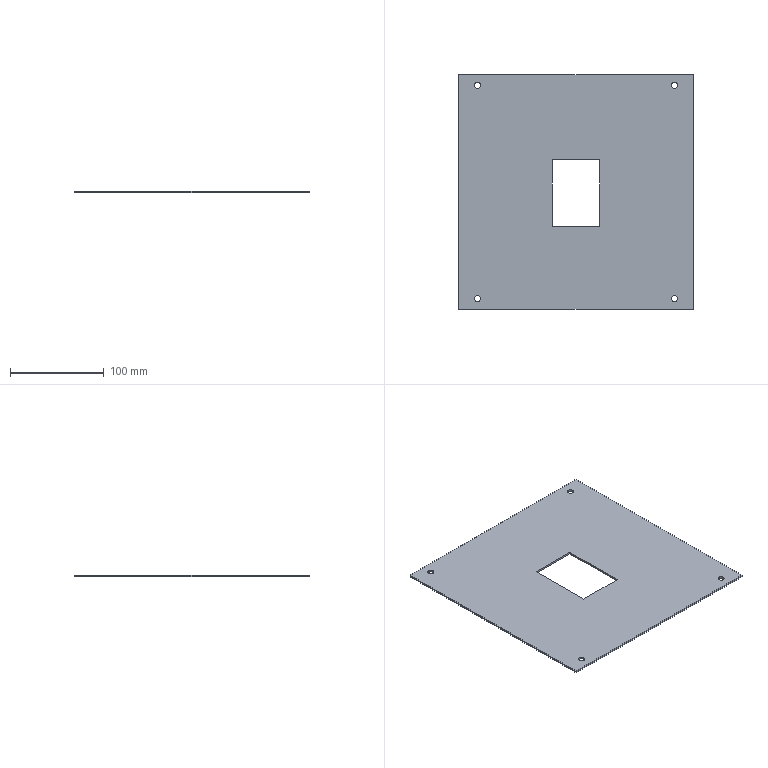Part | SolidWorks | features BaseBody 1 | 1 solid | 18 faces | box 250 x 250 x 2 mm | volume 117542 mm3 | plane 10 | cylinder 8 | commonest cylinder face diameters 6.5 x8
STEP:
#1=CARTESIAN_POINT('',(-108.25,113.5,-2.));
#2=VERTEX_POINT('',#1);
#3=CARTESIAN_POINT('',(-101.75,113.5,-2.));
#4=VERTEX_POINT('',#3);
#5=CARTESIAN_POINT('',(-105.,113.5,-2.));
#6=DIRECTION('',(0.,0.,1.));
#7=DIRECTION('',(1.,0.,0.));
#8=AXIS2_PLACEMENT_3D('',#5,#6,#7);
#9=CIRCLE('',#8,3.25);
#10=EDGE_CURVE('',#2,#4,#9,.T.);
#11=ORIENTED_EDGE('',*,*,#10,.F.);
#12=CARTESIAN_POINT('',(-108.25,113.5,0.));
#13=VERTEX_POINT('',#12);
#14=CARTESIAN_POINT('',(-108.25,113.5,-10.));
#15=DIRECTION('',(0.,0.,1.));
#16=VECTOR('',#15,1000.);
#17=LINE('',#14,#16);
#18=EDGE_CURVE('',#2,#13,#17,.T.);
#19=ORIENTED_EDGE('',*,*,#18,.T.);
#20=CARTESIAN_POINT('',(-101.75,113.5,0.));
#21=VERTEX_POINT('',#20);
#22=CARTESIAN_POINT('',(-105.,113.5,0.));
#23=DIRECTION('',(0.,0.,1.));
#24=DIRECTION('',(1.,0.,0.));
#25=AXIS2_PLACEMENT_3D('',#22,#23,#24);
#26=CIRCLE('',#25,3.25);
#27=EDGE_CURVE('',#13,#21,#26,.T.);
#28=ORIENTED_EDGE('',*,*,#27,.T.);
#29=CARTESIAN_POINT('',(-101.75,113.5,-10.));
#30=DIRECTION('',(0.,0.,1.));
#31=VECTOR('',#30,1000.);
#32=LINE('',#29,#31);
#33=EDGE_CURVE('',#4,#21,#32,.T.);
#34=ORIENTED_EDGE('',*,*,#33,.F.);
#35=EDGE_LOOP('',(#11,#19,#28,#34));
#36=FACE_OUTER_BOUND('',#35,.T.);
#37=CARTESIAN_POINT('',(-105.,113.5,-10.));
#38=DIRECTION('',(0.,0.,1.));
#39=DIRECTION('',(1.,0.,0.));
#40=AXIS2_PLACEMENT_3D('',#37,#38,#39);
#41=CYLINDRICAL_SURFACE('',#40,3.25);
#42=ADVANCED_FACE('',(#36),#41,.F.);
#43=CARTESIAN_POINT('',(101.75,113.5,-2.));
#44=VERTEX_POINT('',#43);
#45=CARTESIAN_POINT('',(108.25,113.5,-2.));
#46=VERTEX_POINT('',#45);
#47=CARTESIAN_POINT('',(105.,113.5,-2.));
#48=DIRECTION('',(0.,0.,1.));
#49=DIRECTION('',(1.,0.,0.));
#50=AXIS2_PLACEMENT_3D('',#47,#48,#49);
#51=CIRCLE('',#50,3.25);
#52=EDGE_CURVE('',#44,#46,#51,.T.);
#53=ORIENTED_EDGE('',*,*,#52,.F.);
#54=CARTESIAN_POINT('',(101.75,113.5,0.));
#55=VERTEX_POINT('',#54);
#56=CARTESIAN_POINT('',(101.75,113.5,-10.));
#57=DIRECTION('',(0.,0.,1.));
#58=VECTOR('',#57,1000.);
#59=LINE('',#56,#58);
#60=EDGE_CURVE('',#44,#55,#59,.T.);
#61=ORIENTED_EDGE('',*,*,#60,.T.);
#62=CARTESIAN_POINT('',(108.25,113.5,0.));
#63=VERTEX_POINT('',#62);
#64=CARTESIAN_POINT('',(105.,113.5,0.));
#65=DIRECTION('',(0.,0.,1.));
#66=DIRECTION('',(1.,0.,0.));
#67=AXIS2_PLACEMENT_3D('',#64,#65,#66);
#68=CIRCLE('',#67,3.25);
#69=EDGE_CURVE('',#55,#63,#68,.T.);
#70=ORIENTED_EDGE('',*,*,#69,.T.);
#71=CARTESIAN_POINT('',(108.25,113.5,-10.));
#72=DIRECTION('',(0.,0.,1.));
#73=VECTOR('',#72,1000.);
#74=LINE('',#71,#73);
#75=EDGE_CURVE('',#46,#63,#74,.T.);
#76=ORIENTED_EDGE('',*,*,#75,.F.);
#77=EDGE_LOOP('',(#53,#61,#70,#76));
#78=FACE_OUTER_BOUND('',#77,.T.);
#79=CARTESIAN_POINT('',(105.,113.5,-10.));
#80=DIRECTION('',(0.,0.,1.));
#81=DIRECTION('',(1.,0.,0.));
#82=AXIS2_PLACEMENT_3D('',#79,#80,#81);
#83=CYLINDRICAL_SURFACE('',#82,3.25);
#84=ADVANCED_FACE('',(#78),#83,.F.);
#85=CARTESIAN_POINT('',(101.75,-113.5,-2.));
#86=VERTEX_POINT('',#85);
#87=CARTESIAN_POINT('',(108.25,-113.5,-2.));
#88=VERTEX_POINT('',#87);
#89=CARTESIAN_POINT('',(105.,-113.5,-2.));
#90=DIRECTION('',(0.,0.,1.));
#91=DIRECTION('',(1.,0.,0.));
#92=AXIS2_PLACEMENT_3D('',#89,#90,#91);
#93=CIRCLE('',#92,3.25);
#94=EDGE_CURVE('',#86,#88,#93,.T.);
#95=ORIENTED_EDGE('',*,*,#94,.F.);
#96=CARTESIAN_POINT('',(101.75,-113.5,0.));
#97=VERTEX_POINT('',#96);
#98=CARTESIAN_POINT('',(101.75,-113.5,-10.));
#99=DIRECTION('',(0.,0.,1.));
#100=VECTOR('',#99,1000.);
#101=LINE('',#98,#100);
#102=EDGE_CURVE('',#86,#97,#101,.T.);
#103=ORIENTED_EDGE('',*,*,#102,.T.);
#104=CARTESIAN_POINT('',(108.25,-113.5,0.));
#105=VERTEX_POINT('',#104);
#106=CARTESIAN_POINT('',(105.,-113.5,0.));
#107=DIRECTION('',(0.,0.,1.));
#108=DIRECTION('',(1.,0.,0.));
#109=AXIS2_PLACEMENT_3D('',#106,#107,#108);
#110=CIRCLE('',#109,3.25);
#111=EDGE_CURVE('',#97,#105,#110,.T.);
#112=ORIENTED_EDGE('',*,*,#111,.T.);
#113=CARTESIAN_POINT('',(108.25,-113.5,-10.));
#114=DIRECTION('',(0.,0.,1.));
#115=VECTOR('',#114,1000.);
#116=LINE('',#113,#115);
#117=EDGE_CURVE('',#88,#105,#116,.T.);
#118=ORIENTED_EDGE('',*,*,#117,.F.);
#119=EDGE_LOOP('',(#95,#103,#112,#118));
#120=FACE_OUTER_BOUND('',#119,.T.);
#121=CARTESIAN_POINT('',(105.,-113.5,-10.));
#122=DIRECTION('',(0.,0.,1.));
#123=DIRECTION('',(1.,0.,0.));
#124=AXIS2_PLACEMENT_3D('',#121,#122,#123);
#125=CYLINDRICAL_SURFACE('',#124,3.25);
#126=ADVANCED_FACE('',(#120),#125,.F.);
#127=CARTESIAN_POINT('',(-108.25,-113.5,-2.));
#128=VERTEX_POINT('',#127);
#129=CARTESIAN_POINT('',(-101.75,-113.5,-2.));
#130=VERTEX_POINT('',#129);
#131=CARTESIAN_POINT('',(-105.,-113.5,-2.));
#132=DIRECTION('',(0.,0.,1.));
#133=DIRECTION('',(1.,0.,0.));
#134=AXIS2_PLACEMENT_3D('',#131,#132,#133);
#135=CIRCLE('',#134,3.25);
#136=EDGE_CURVE('',#128,#130,#135,.T.);
#137=ORIENTED_EDGE('',*,*,#136,.F.);
#138=CARTESIAN_POINT('',(-108.25,-113.5,0.));
#139=VERTEX_POINT('',#138);
#140=CARTESIAN_POINT('',(-108.25,-113.5,-10.));
#141=DIRECTION('',(0.,0.,1.));
#142=VECTOR('',#141,1000.);
#143=LINE('',#140,#142);
#144=EDGE_CURVE('',#128,#139,#143,.T.);
#145=ORIENTED_EDGE('',*,*,#144,.T.);
#146=CARTESIAN_POINT('',(-101.75,-113.5,0.));
#147=VERTEX_POINT('',#146);
#148=CARTESIAN_POINT('',(-105.,-113.5,0.));
#149=DIRECTION('',(0.,0.,1.));
#150=DIRECTION('',(1.,0.,0.));
#151=AXIS2_PLACEMENT_3D('',#148,#149,#150);
#152=CIRCLE('',#151,3.25);
#153=EDGE_CURVE('',#139,#147,#152,.T.);
#154=ORIENTED_EDGE('',*,*,#153,.T.);
#155=CARTESIAN_POINT('',(-101.75,-113.5,-10.));
#156=DIRECTION('',(0.,0.,1.));
#157=VECTOR('',#156,1000.);
#158=LINE('',#155,#157);
#159=EDGE_CURVE('',#130,#147,#158,.T.);
#160=ORIENTED_EDGE('',*,*,#159,.F.);
#161=EDGE_LOOP('',(#137,#145,#154,#160));
#162=FACE_OUTER_BOUND('',#161,.T.);
#163=CARTESIAN_POINT('',(-105.,-113.5,-10.));
#164=DIRECTION('',(0.,0.,1.));
#165=DIRECTION('',(1.,0.,0.));
#166=AXIS2_PLACEMENT_3D('',#163,#164,#165);
#167=CYLINDRICAL_SURFACE('',#166,3.25);
#168=ADVANCED_FACE('',(#162),#167,.F.);
#169=CARTESIAN_POINT('',(-125.,125.,0.));
#170=VERTEX_POINT('',#169);
#171=CARTESIAN_POINT('',(125.,125.,0.));
#172=VERTEX_POINT('',#171);
#173=CARTESIAN_POINT('',(0.,125.,0.));
#174=DIRECTION('',(1.,0.,0.));
#175=VECTOR('',#174,1000.);
#176=LINE('',#173,#175);
#177=EDGE_CURVE('',#170,#172,#176,.T.);
#178=ORIENTED_EDGE('',*,*,#177,.F.);
#179=CARTESIAN_POINT('',(-125.,-125.,0.));
#180=VERTEX_POINT('',#179);
#181=CARTESIAN_POINT('',(-125.,0.,0.));
#182=DIRECTION('',(0.,1.,0.));
#183=VECTOR('',#182,1000.);
#184=LINE('',#181,#183);
#185=EDGE_CURVE('',#180,#170,#184,.T.);
#186=ORIENTED_EDGE('',*,*,#185,.F.);
#187=CARTESIAN_POINT('',(125.,-125.,0.));
#188=VERTEX_POINT('',#187);
#189=CARTESIAN_POINT('',(0.,-125.,0.));
#190=DIRECTION('',(-1.,0.,0.));
#191=VECTOR('',#190,1000.);
#192=LINE('',#189,#191);
#193=EDGE_CURVE('',#188,#180,#192,.T.);
#194=ORIENTED_EDGE('',*,*,#193,.F.);
#195=CARTESIAN_POINT('',(125.,0.,0.));
#196=DIRECTION('',(0.,-1.,0.));
#197=VECTOR('',#196,1000.);
#198=LINE('',#195,#197);
#199=EDGE_CURVE('',#172,#188,#198,.T.);
#200=ORIENTED_EDGE('',*,*,#199,.F.);
#201=EDGE_LOOP('',(#178,#186,#194,#200));
#202=FACE_OUTER_BOUND('',#201,.T.);
#203=CARTESIAN_POINT('',(-105.,113.5,0.));
#204=DIRECTION('',(0.,0.,1.));
#205=DIRECTION('',(1.,0.,0.));
#206=AXIS2_PLACEMENT_3D('',#203,#204,#205);
#207=CIRCLE('',#206,3.25);
#208=EDGE_CURVE('',#21,#13,#207,.T.);
#209=ORIENTED_EDGE('',*,*,#208,.F.);
#210=ORIENTED_EDGE('',*,*,#27,.F.);
#211=EDGE_LOOP('',(#209,#210));
#212=FACE_BOUND('',#211,.T.);
#213=CARTESIAN_POINT('',(105.,113.5,0.));
#214=DIRECTION('',(0.,0.,1.));
#215=DIRECTION('',(1.,0.,0.));
#216=AXIS2_PLACEMENT_3D('',#213,#214,#215);
#217=CIRCLE('',#216,3.25);
#218=EDGE_CURVE('',#63,#55,#217,.T.);
#219=ORIENTED_EDGE('',*,*,#218,.F.);
#220=ORIENTED_EDGE('',*,*,#69,.F.);
#221=EDGE_LOOP('',(#219,#220));
#222=FACE_BOUND('',#221,.T.);
#223=CARTESIAN_POINT('',(105.,-113.5,0.));
#224=DIRECTION('',(0.,0.,1.));
#225=DIRECTION('',(1.,0.,0.));
#226=AXIS2_PLACEMENT_3D('',#223,#224,#225);
#227=CIRCLE('',#226,3.25);
#228=EDGE_CURVE('',#105,#97,#227,.T.);
#229=ORIENTED_EDGE('',*,*,#228,.F.);
#230=ORIENTED_EDGE('',*,*,#111,.F.);
#231=EDGE_LOOP('',(#229,#230));
#232=FACE_BOUND('',#231,.T.);
#233=CARTESIAN_POINT('',(-105.,-113.5,0.));
#234=DIRECTION('',(0.,0.,1.));
#235=DIRECTION('',(1.,0.,0.));
#236=AXIS2_PLACEMENT_3D('',#233,#234,#235);
#237=CIRCLE('',#236,3.25);
#238=EDGE_CURVE('',#147,#139,#237,.T.);
#239=ORIENTED_EDGE('',*,*,#238,.F.);
#240=ORIENTED_EDGE('',*,*,#153,.F.);
#241=EDGE_LOOP('',(#239,#240));
#242=FACE_BOUND('',#241,.T.);
#243=CARTESIAN_POINT('',(25.25,-36.805,0.));
#244=VERTEX_POINT('',#243);
#245=CARTESIAN_POINT('',(25.25,34.405,0.));
#246=VERTEX_POINT('',#245);
#247=CARTESIAN_POINT('',(25.25,0.,0.));
#248=DIRECTION('',(0.,1.,0.));
#249=VECTOR('',#248,1000.);
#250=LINE('',#247,#249);
#251=EDGE_CURVE('',#244,#246,#250,.T.);
#252=ORIENTED_EDGE('',*,*,#251,.F.);
#253=CARTESIAN_POINT('',(-25.25,-36.805,0.));
#254=VERTEX_POINT('',#253);
#255=CARTESIAN_POINT('',(0.,-36.805,0.));
#256=DIRECTION('',(1.,0.,0.));
#257=VECTOR('',#256,1000.);
#258=LINE('',#255,#257);
#259=EDGE_CURVE('',#254,#244,#258,.T.);
#260=ORIENTED_EDGE('',*,*,#259,.F.);
#261=CARTESIAN_POINT('',(-25.25,34.405,0.));
#262=VERTEX_POINT('',#261);
#263=CARTESIAN_POINT('',(-25.25,0.,0.));
#264=DIRECTION('',(0.,-1.,0.));
#265=VECTOR('',#264,1000.);
#266=LINE('',#263,#265);
#267=EDGE_CURVE('',#262,#254,#266,.T.);
#268=ORIENTED_EDGE('',*,*,#267,.F.);
#269=CARTESIAN_POINT('',(0.,34.405,0.));
#270=DIRECTION('',(-1.,0.,0.));
#271=VECTOR('',#270,1000.);
#272=LINE('',#269,#271);
#273=EDGE_CURVE('',#246,#262,#272,.T.);
#274=ORIENTED_EDGE('',*,*,#273,.F.);
#275=EDGE_LOOP('',(#252,#260,#268,#274));
#276=FACE_BOUND('',#275,.T.);
#277=CARTESIAN_POINT('',(0.,0.,0.));
#278=DIRECTION('',(0.,0.,-1.));
#279=DIRECTION('',(-1.,0.,0.));
#280=AXIS2_PLACEMENT_3D('',#277,#278,#279);
#281=PLANE('',#280);
#282=ADVANCED_FACE('',(#202,#212,#222,#232,#242,#276),#281,.F.);
#283=CARTESIAN_POINT('',(125.,-125.,-2.));
#284=VERTEX_POINT('',#283);
#285=CARTESIAN_POINT('',(125.,125.,-2.));
#286=VERTEX_POINT('',#285);
#287=CARTESIAN_POINT('',(125.,-125.,-2.));
#288=DIRECTION('',(0.,1.,0.));
#289=VECTOR('',#288,1000.);
#290=LINE('',#287,#289);
#291=EDGE_CURVE('',#284,#286,#290,.T.);
#292=ORIENTED_EDGE('',*,*,#291,.T.);
#293=CARTESIAN_POINT('',(125.,125.,-2.));
#294=DIRECTION('',(0.,0.,1.));
#295=VECTOR('',#294,1000.);
#296=LINE('',#293,#295);
#297=EDGE_CURVE('',#286,#172,#296,.T.);
#298=ORIENTED_EDGE('',*,*,#297,.T.);
#299=ORIENTED_EDGE('',*,*,#199,.T.);
#300=CARTESIAN_POINT('',(125.,-125.,-2.));
#301=DIRECTION('',(0.,0.,-1.));
#302=VECTOR('',#301,1000.);
#303=LINE('',#300,#302);
#304=EDGE_CURVE('',#188,#284,#303,.T.);
#305=ORIENTED_EDGE('',*,*,#304,.T.);
#306=EDGE_LOOP('',(#292,#298,#299,#305));
#307=FACE_OUTER_BOUND('',#306,.T.);
#308=CARTESIAN_POINT('',(125.,-125.,-2.));
#309=DIRECTION('',(1.,0.,0.));
#310=DIRECTION('',(0.,0.,-1.));
#311=AXIS2_PLACEMENT_3D('',#308,#309,#310);
#312=PLANE('',#311);
#313=ADVANCED_FACE('',(#307),#312,.T.);
#314=CARTESIAN_POINT('',(-125.,125.,-2.));
#315=VERTEX_POINT('',#314);
#316=CARTESIAN_POINT('',(-125.,125.,-2.));
#317=DIRECTION('',(-1.,0.,0.));
#318=VECTOR('',#317,1000.);
#319=LINE('',#316,#318);
#320=EDGE_CURVE('',#286,#315,#319,.T.);
#321=ORIENTED_EDGE('',*,*,#320,.T.);
#322=CARTESIAN_POINT('',(-125.,125.,-2.));
#323=DIRECTION('',(0.,0.,1.));
#324=VECTOR('',#323,1000.);
#325=LINE('',#322,#324);
#326=EDGE_CURVE('',#315,#170,#325,.T.);
#327=ORIENTED_EDGE('',*,*,#326,.T.);
#328=ORIENTED_EDGE('',*,*,#177,.T.);
#329=ORIENTED_EDGE('',*,*,#297,.F.);
#330=EDGE_LOOP('',(#321,#327,#328,#329));
#331=FACE_OUTER_BOUND('',#330,.T.);
#332=CARTESIAN_POINT('',(-125.,125.,-2.));
#333=DIRECTION('',(0.,1.,0.));
#334=DIRECTION('',(0.,0.,1.));
#335=AXIS2_PLACEMENT_3D('',#332,#333,#334);
#336=PLANE('',#335);
#337=ADVANCED_FACE('',(#331),#336,.T.);
#338=CARTESIAN_POINT('',(-125.,-125.,-2.));
#339=VERTEX_POINT('',#338);
#340=CARTESIAN_POINT('',(-125.,-125.,-2.));
#341=DIRECTION('',(0.,-1.,0.));
#342=VECTOR('',#341,1000.);
#343=LINE('',#340,#342);
#344=EDGE_CURVE('',#315,#339,#343,.T.);
#345=ORIENTED_EDGE('',*,*,#344,.T.);
#346=CARTESIAN_POINT('',(-125.,-125.,-2.));
#347=DIRECTION('',(0.,0.,1.));
#348=VECTOR('',#347,1000.);
#349=LINE('',#346,#348);
#350=EDGE_CURVE('',#339,#180,#349,.T.);
#351=ORIENTED_EDGE('',*,*,#350,.T.);
#352=ORIENTED_EDGE('',*,*,#185,.T.);
#353=ORIENTED_EDGE('',*,*,#326,.F.);
#354=EDGE_LOOP('',(#345,#351,#352,#353));
#355=FACE_OUTER_BOUND('',#354,.T.);
#356=CARTESIAN_POINT('',(-125.,-125.,-2.));
#357=DIRECTION('',(-1.,0.,0.));
#358=DIRECTION('',(0.,0.,1.));
#359=AXIS2_PLACEMENT_3D('',#356,#357,#358);
#360=PLANE('',#359);
#361=ADVANCED_FACE('',(#355),#360,.T.);
#362=CARTESIAN_POINT('',(-125.,-125.,-2.));
#363=DIRECTION('',(1.,0.,0.));
#364=VECTOR('',#363,1000.);
#365=LINE('',#362,#364);
#366=EDGE_CURVE('',#339,#284,#365,.T.);
#367=ORIENTED_EDGE('',*,*,#366,.T.);
#368=ORIENTED_EDGE('',*,*,#304,.F.);
#369=ORIENTED_EDGE('',*,*,#193,.T.);
#370=ORIENTED_EDGE('',*,*,#350,.F.);
#371=EDGE_LOOP('',(#367,#368,#369,#370));
#372=FACE_OUTER_BOUND('',#371,.T.);
#373=CARTESIAN_POINT('',(-125.,-125.,-2.));
#374=DIRECTION('',(0.,-1.,0.));
#375=DIRECTION('',(0.,0.,-1.));
#376=AXIS2_PLACEMENT_3D('',#373,#374,#375);
#377=PLANE('',#376);
#378=ADVANCED_FACE('',(#372),#377,.T.);
#379=ORIENTED_EDGE('',*,*,#18,.F.);
#380=CARTESIAN_POINT('',(-105.,113.5,-2.));
#381=DIRECTION('',(0.,0.,1.));
#382=DIRECTION('',(1.,0.,0.));
#383=AXIS2_PLACEMENT_3D('',#380,#381,#382);
#384=CIRCLE('',#383,3.25);
#385=EDGE_CURVE('',#4,#2,#384,.T.);
#386=ORIENTED_EDGE('',*,*,#385,.F.);
#387=ORIENTED_EDGE('',*,*,#33,.T.);
#388=ORIENTED_EDGE('',*,*,#208,.T.);
#389=EDGE_LOOP('',(#379,#386,#387,#388));
#390=FACE_OUTER_BOUND('',#389,.T.);
#391=CARTESIAN_POINT('',(-105.,113.5,-10.));
#392=DIRECTION('',(0.,0.,1.));
#393=DIRECTION('',(1.,0.,0.));
#394=AXIS2_PLACEMENT_3D('',#391,#392,#393);
#395=CYLINDRICAL_SURFACE('',#394,3.25);
#396=ADVANCED_FACE('',(#390),#395,.F.);
#397=ORIENTED_EDGE('',*,*,#60,.F.);
#398=CARTESIAN_POINT('',(105.,113.5,-2.));
#399=DIRECTION('',(0.,0.,1.));
#400=DIRECTION('',(1.,0.,0.));
#401=AXIS2_PLACEMENT_3D('',#398,#399,#400);
#402=CIRCLE('',#401,3.25);
#403=EDGE_CURVE('',#46,#44,#402,.T.);
#404=ORIENTED_EDGE('',*,*,#403,.F.);
#405=ORIENTED_EDGE('',*,*,#75,.T.);
#406=ORIENTED_EDGE('',*,*,#218,.T.);
#407=EDGE_LOOP('',(#397,#404,#405,#406));
#408=FACE_OUTER_BOUND('',#407,.T.);
#409=CARTESIAN_POINT('',(105.,113.5,-10.));
#410=DIRECTION('',(0.,0.,1.));
#411=DIRECTION('',(1.,0.,0.));
#412=AXIS2_PLACEMENT_3D('',#409,#410,#411);
#413=CYLINDRICAL_SURFACE('',#412,3.25);
#414=ADVANCED_FACE('',(#408),#413,.F.);
#415=ORIENTED_EDGE('',*,*,#102,.F.);
#416=CARTESIAN_POINT('',(105.,-113.5,-2.));
#417=DIRECTION('',(0.,0.,1.));
#418=DIRECTION('',(1.,0.,0.));
#419=AXIS2_PLACEMENT_3D('',#416,#417,#418);
#420=CIRCLE('',#419,3.25);
#421=EDGE_CURVE('',#88,#86,#420,.T.);
#422=ORIENTED_EDGE('',*,*,#421,.F.);
#423=ORIENTED_EDGE('',*,*,#117,.T.);
#424=ORIENTED_EDGE('',*,*,#228,.T.);
#425=EDGE_LOOP('',(#415,#422,#423,#424));
#426=FACE_OUTER_BOUND('',#425,.T.);
#427=CARTESIAN_POINT('',(105.,-113.5,-10.));
#428=DIRECTION('',(0.,0.,1.));
#429=DIRECTION('',(1.,0.,0.));
#430=AXIS2_PLACEMENT_3D('',#427,#428,#429);
#431=CYLINDRICAL_SURFACE('',#430,3.25);
#432=ADVANCED_FACE('',(#426),#431,.F.);
#433=ORIENTED_EDGE('',*,*,#144,.F.);
#434=CARTESIAN_POINT('',(-105.,-113.5,-2.));
#435=DIRECTION('',(0.,0.,1.));
#436=DIRECTION('',(1.,0.,0.));
#437=AXIS2_PLACEMENT_3D('',#434,#435,#436);
#438=CIRCLE('',#437,3.25);
#439=EDGE_CURVE('',#130,#128,#438,.T.);
#440=ORIENTED_EDGE('',*,*,#439,.F.);
#441=ORIENTED_EDGE('',*,*,#159,.T.);
#442=ORIENTED_EDGE('',*,*,#238,.T.);
#443=EDGE_LOOP('',(#433,#440,#441,#442));
#444=FACE_OUTER_BOUND('',#443,.T.);
#445=CARTESIAN_POINT('',(-105.,-113.5,-10.));
#446=DIRECTION('',(0.,0.,1.));
#447=DIRECTION('',(1.,0.,0.));
#448=AXIS2_PLACEMENT_3D('',#445,#446,#447);
#449=CYLINDRICAL_SURFACE('',#448,3.25);
#450=ADVANCED_FACE('',(#444),#449,.F.);
#451=CARTESIAN_POINT('',(25.25,34.405,-2.));
#452=VERTEX_POINT('',#451);
#453=CARTESIAN_POINT('',(-25.25,34.405,-2.));
#454=VERTEX_POINT('',#453);
#455=CARTESIAN_POINT('',(25.25,34.405,-2.));
#456=DIRECTION('',(-1.,0.,0.));
#457=VECTOR('',#456,1000.);
#458=LINE('',#455,#457);
#459=EDGE_CURVE('',#452,#454,#458,.T.);
#460=ORIENTED_EDGE('',*,*,#459,.F.);
#461=CARTESIAN_POINT('',(25.25,34.405,8.));
#462=DIRECTION('',(0.,0.,-1.));
#463=VECTOR('',#462,1000.);
#464=LINE('',#461,#463);
#465=EDGE_CURVE('',#246,#452,#464,.T.);
#466=ORIENTED_EDGE('',*,*,#465,.F.);
#467=ORIENTED_EDGE('',*,*,#273,.T.);
#468=CARTESIAN_POINT('',(-25.25,34.405,8.));
#469=DIRECTION('',(0.,0.,1.));
#470=VECTOR('',#469,1000.);
#471=LINE('',#468,#470);
#472=EDGE_CURVE('',#454,#262,#471,.T.);
#473=ORIENTED_EDGE('',*,*,#472,.F.);
#474=EDGE_LOOP('',(#460,#466,#467,#473));
#475=FACE_OUTER_BOUND('',#474,.T.);
#476=CARTESIAN_POINT('',(25.25,34.405,8.));
#477=DIRECTION('',(0.,1.,0.));
#478=DIRECTION('',(0.,0.,1.));
#479=AXIS2_PLACEMENT_3D('',#476,#477,#478);
#480=PLANE('',#479);
#481=ADVANCED_FACE('',(#475),#480,.F.);
#482=CARTESIAN_POINT('',(25.25,-36.805,-2.));
#483=VERTEX_POINT('',#482);
#484=CARTESIAN_POINT('',(25.25,34.405,-2.));
#485=DIRECTION('',(0.,1.,0.));
#486=VECTOR('',#485,1000.);
#487=LINE('',#484,#486);
#488=EDGE_CURVE('',#483,#452,#487,.T.);
#489=ORIENTED_EDGE('',*,*,#488,.F.);
#490=CARTESIAN_POINT('',(25.25,-36.805,8.));
#491=DIRECTION('',(0.,0.,-1.));
#492=VECTOR('',#491,1000.);
#493=LINE('',#490,#492);
#494=EDGE_CURVE('',#244,#483,#493,.T.);
#495=ORIENTED_EDGE('',*,*,#494,.F.);
#496=ORIENTED_EDGE('',*,*,#251,.T.);
#497=ORIENTED_EDGE('',*,*,#465,.T.);
#498=EDGE_LOOP('',(#489,#495,#496,#497));
#499=FACE_OUTER_BOUND('',#498,.T.);
#500=CARTESIAN_POINT('',(25.25,34.405,8.));
#501=DIRECTION('',(1.,0.,0.));
#502=DIRECTION('',(0.,0.,-1.));
#503=AXIS2_PLACEMENT_3D('',#500,#501,#502);
#504=PLANE('',#503);
#505=ADVANCED_FACE('',(#499),#504,.F.);
#506=CARTESIAN_POINT('',(-25.25,-36.805,-2.));
#507=VERTEX_POINT('',#506);
#508=CARTESIAN_POINT('',(25.25,-36.805,-2.));
#509=DIRECTION('',(1.,0.,0.));
#510=VECTOR('',#509,1000.);
#511=LINE('',#508,#510);
#512=EDGE_CURVE('',#507,#483,#511,.T.);
#513=ORIENTED_EDGE('',*,*,#512,.F.);
#514=CARTESIAN_POINT('',(-25.25,-36.805,8.));
#515=DIRECTION('',(0.,0.,-1.));
#516=VECTOR('',#515,1000.);
#517=LINE('',#514,#516);
#518=EDGE_CURVE('',#254,#507,#517,.T.);
#519=ORIENTED_EDGE('',*,*,#518,.F.);
#520=ORIENTED_EDGE('',*,*,#259,.T.);
#521=ORIENTED_EDGE('',*,*,#494,.T.);
#522=EDGE_LOOP('',(#513,#519,#520,#521));
#523=FACE_OUTER_BOUND('',#522,.T.);
#524=CARTESIAN_POINT('',(25.25,-36.805,8.));
#525=DIRECTION('',(0.,-1.,0.));
#526=DIRECTION('',(1.,0.,0.));
#527=AXIS2_PLACEMENT_3D('',#524,#525,#526);
#528=PLANE('',#527);
#529=ADVANCED_FACE('',(#523),#528,.F.);
#530=CARTESIAN_POINT('',(-25.25,34.405,-2.));
#531=DIRECTION('',(0.,-1.,0.));
#532=VECTOR('',#531,1000.);
#533=LINE('',#530,#532);
#534=EDGE_CURVE('',#454,#507,#533,.T.);
#535=ORIENTED_EDGE('',*,*,#534,.F.);
#536=ORIENTED_EDGE('',*,*,#472,.T.);
#537=ORIENTED_EDGE('',*,*,#267,.T.);
#538=ORIENTED_EDGE('',*,*,#518,.T.);
#539=EDGE_LOOP('',(#535,#536,#537,#538));
#540=FACE_OUTER_BOUND('',#539,.T.);
#541=CARTESIAN_POINT('',(-25.25,34.405,8.));
#542=DIRECTION('',(-1.,0.,0.));
#543=DIRECTION('',(0.,0.,1.));
#544=AXIS2_PLACEMENT_3D('',#541,#542,#543);
#545=PLANE('',#544);
#546=ADVANCED_FACE('',(#540),#545,.F.);
#547=ORIENTED_EDGE('',*,*,#344,.F.);
#548=ORIENTED_EDGE('',*,*,#320,.F.);
#549=ORIENTED_EDGE('',*,*,#291,.F.);
#550=ORIENTED_EDGE('',*,*,#366,.F.);
#551=EDGE_LOOP('',(#547,#548,#549,#550));
#552=FACE_OUTER_BOUND('',#551,.T.);
#553=ORIENTED_EDGE('',*,*,#385,.T.);
#554=ORIENTED_EDGE('',*,*,#10,.T.);
#555=EDGE_LOOP('',(#553,#554));
#556=FACE_BOUND('',#555,.T.);
#557=ORIENTED_EDGE('',*,*,#403,.T.);
#558=ORIENTED_EDGE('',*,*,#52,.T.);
#559=EDGE_LOOP('',(#557,#558));
#560=FACE_BOUND('',#559,.T.);
#561=ORIENTED_EDGE('',*,*,#421,.T.);
#562=ORIENTED_EDGE('',*,*,#94,.T.);
#563=EDGE_LOOP('',(#561,#562));
#564=FACE_BOUND('',#563,.T.);
#565=ORIENTED_EDGE('',*,*,#439,.T.);
#566=ORIENTED_EDGE('',*,*,#136,.T.);
#567=EDGE_LOOP('',(#565,#566));
#568=FACE_BOUND('',#567,.T.);
#569=ORIENTED_EDGE('',*,*,#534,.T.);
#570=ORIENTED_EDGE('',*,*,#512,.T.);
#571=ORIENTED_EDGE('',*,*,#488,.T.);
#572=ORIENTED_EDGE('',*,*,#459,.T.);
#573=EDGE_LOOP('',(#569,#570,#571,#572));
#574=FACE_BOUND('',#573,.T.);
#575=CARTESIAN_POINT('',(0.,0.,-2.));
#576=DIRECTION('',(0.,0.,-1.));
#577=DIRECTION('',(-1.,0.,0.));
#578=AXIS2_PLACEMENT_3D('',#575,#576,#577);
#579=PLANE('',#578);
#580=ADVANCED_FACE('',(#552,#556,#560,#564,#568,#574),#579,.T.);
#581=CLOSED_SHELL('',(#42,#84,#126,#168,#282,#313,#337,#361,#378,#396,#414,#432,#450,#481,#505,#529,#546,#580));
#582=MANIFOLD_SOLID_BREP('',#581);
#583=CARTESIAN_POINT('',(0.,0.,0.));
#584=DIRECTION('',(0.,0.,1.));
#585=DIRECTION('',(1.,0.,0.));
#586=AXIS2_PLACEMENT_3D('',#583,#584,#585);
#587=(LENGTH_UNIT()NAMED_UNIT(*)SI_UNIT(.MILLI.,.METRE.));
#588=UNCERTAINTY_MEASURE_WITH_UNIT(LENGTH_MEASURE(0.00001),#587,'','');
#589=(NAMED_UNIT(*)PLANE_ANGLE_UNIT()SI_UNIT($,.RADIAN.));
#590=(NAMED_UNIT(*)SI_UNIT($,.STERADIAN.)SOLID_ANGLE_UNIT());
#591=(GEOMETRIC_REPRESENTATION_CONTEXT(3)GLOBAL_UNCERTAINTY_ASSIGNED_CONTEXT((#588))GLOBAL_UNIT_ASSIGNED_CONTEXT((#587,#589,#590))REPRESENTATION_CONTEXT('',''));
#592=ADVANCED_BREP_SHAPE_REPRESENTATION('',(#582,#586),#591);